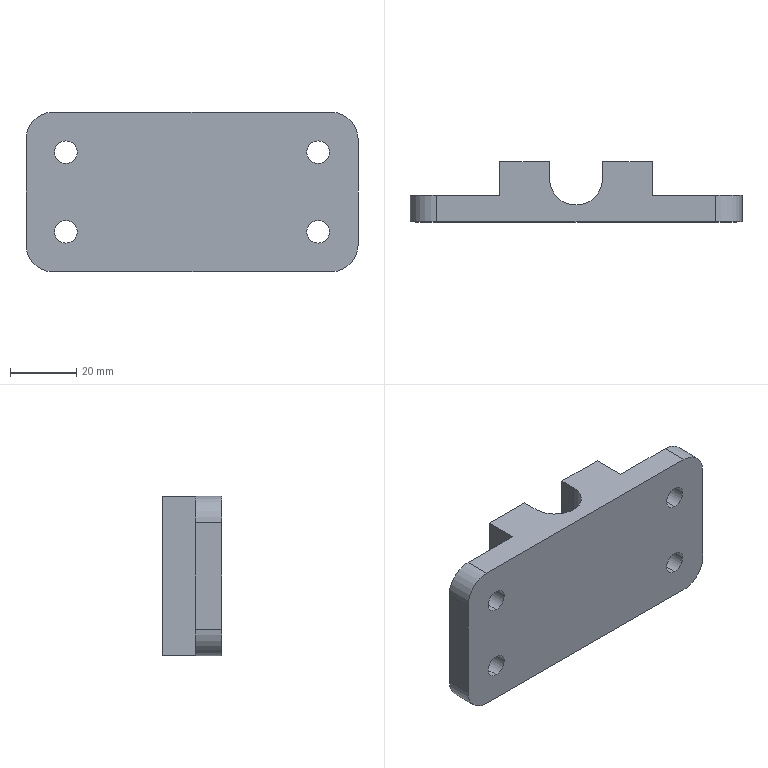Part | SolidWorks | features HoleWzd 2, ICE 2, Extrusion 1, Fillet 1 | 1 solid | 42 faces | box 100 x 18 x 48 mm | volume 49859 mm3 | cylinder 21 | plane 13 | cone 8 | commonest cylinder face diameters 3.3 x8 6.8 x8 16 x5
STEP:
#1=CARTESIAN_POINT('',(-38.,0.,-15.4));
#2=VERTEX_POINT('',#1);
#3=CARTESIAN_POINT('',(-38.,0.,-8.6));
#4=VERTEX_POINT('',#3);
#5=CARTESIAN_POINT('',(-38.,0.,-12.));
#6=DIRECTION('',(0.,1.,0.));
#7=DIRECTION('',(0.,0.,1.));
#8=AXIS2_PLACEMENT_3D('',#5,#6,#7);
#9=CIRCLE('',#8,3.4);
#10=EDGE_CURVE('',#2,#4,#9,.T.);
#11=ORIENTED_EDGE('',*,*,#10,.F.);
#12=CARTESIAN_POINT('',(-38.,8.,-15.4));
#13=VERTEX_POINT('',#12);
#14=CARTESIAN_POINT('',(-38.,8.,-15.4));
#15=DIRECTION('',(0.,1.,0.));
#16=VECTOR('',#15,1000.);
#17=LINE('',#14,#16);
#18=EDGE_CURVE('',#2,#13,#17,.T.);
#19=ORIENTED_EDGE('',*,*,#18,.T.);
#20=CARTESIAN_POINT('',(-38.,8.,-8.6));
#21=VERTEX_POINT('',#20);
#22=CARTESIAN_POINT('',(-38.,8.,-12.));
#23=DIRECTION('',(0.,1.,0.));
#24=DIRECTION('',(0.,0.,1.));
#25=AXIS2_PLACEMENT_3D('',#22,#23,#24);
#26=CIRCLE('',#25,3.4);
#27=EDGE_CURVE('',#13,#21,#26,.T.);
#28=ORIENTED_EDGE('',*,*,#27,.T.);
#29=CARTESIAN_POINT('',(-38.,8.,-8.6));
#30=DIRECTION('',(0.,1.,0.));
#31=VECTOR('',#30,1000.);
#32=LINE('',#29,#31);
#33=EDGE_CURVE('',#4,#21,#32,.T.);
#34=ORIENTED_EDGE('',*,*,#33,.F.);
#35=EDGE_LOOP('',(#11,#19,#28,#34));
#36=FACE_OUTER_BOUND('',#35,.T.);
#37=CARTESIAN_POINT('',(-38.,8.,-12.));
#38=DIRECTION('',(0.,1.,0.));
#39=DIRECTION('',(0.,0.,1.));
#40=AXIS2_PLACEMENT_3D('',#37,#38,#39);
#41=CYLINDRICAL_SURFACE('',#40,3.4);
#42=ADVANCED_FACE('',(#36),#41,.F.);
#43=CARTESIAN_POINT('',(-38.,0.,8.6));
#44=VERTEX_POINT('',#43);
#45=CARTESIAN_POINT('',(-38.,0.,15.4));
#46=VERTEX_POINT('',#45);
#47=CARTESIAN_POINT('',(-38.,0.,12.));
#48=DIRECTION('',(0.,1.,0.));
#49=DIRECTION('',(0.,0.,1.));
#50=AXIS2_PLACEMENT_3D('',#47,#48,#49);
#51=CIRCLE('',#50,3.4);
#52=EDGE_CURVE('',#44,#46,#51,.T.);
#53=ORIENTED_EDGE('',*,*,#52,.F.);
#54=CARTESIAN_POINT('',(-38.,8.,8.6));
#55=VERTEX_POINT('',#54);
#56=CARTESIAN_POINT('',(-38.,8.,8.6));
#57=DIRECTION('',(0.,1.,0.));
#58=VECTOR('',#57,1000.);
#59=LINE('',#56,#58);
#60=EDGE_CURVE('',#44,#55,#59,.T.);
#61=ORIENTED_EDGE('',*,*,#60,.T.);
#62=CARTESIAN_POINT('',(-38.,8.,15.4));
#63=VERTEX_POINT('',#62);
#64=CARTESIAN_POINT('',(-38.,8.,12.));
#65=DIRECTION('',(0.,1.,0.));
#66=DIRECTION('',(0.,0.,1.));
#67=AXIS2_PLACEMENT_3D('',#64,#65,#66);
#68=CIRCLE('',#67,3.4);
#69=EDGE_CURVE('',#55,#63,#68,.T.);
#70=ORIENTED_EDGE('',*,*,#69,.T.);
#71=CARTESIAN_POINT('',(-38.,8.,15.4));
#72=DIRECTION('',(0.,1.,0.));
#73=VECTOR('',#72,1000.);
#74=LINE('',#71,#73);
#75=EDGE_CURVE('',#46,#63,#74,.T.);
#76=ORIENTED_EDGE('',*,*,#75,.F.);
#77=EDGE_LOOP('',(#53,#61,#70,#76));
#78=FACE_OUTER_BOUND('',#77,.T.);
#79=CARTESIAN_POINT('',(-38.,8.,12.));
#80=DIRECTION('',(0.,1.,0.));
#81=DIRECTION('',(0.,0.,1.));
#82=AXIS2_PLACEMENT_3D('',#79,#80,#81);
#83=CYLINDRICAL_SURFACE('',#82,3.4);
#84=ADVANCED_FACE('',(#78),#83,.F.);
#85=CARTESIAN_POINT('',(38.,0.,8.6));
#86=VERTEX_POINT('',#85);
#87=CARTESIAN_POINT('',(38.,0.,15.4));
#88=VERTEX_POINT('',#87);
#89=CARTESIAN_POINT('',(38.,0.,12.));
#90=DIRECTION('',(0.,1.,0.));
#91=DIRECTION('',(0.,0.,1.));
#92=AXIS2_PLACEMENT_3D('',#89,#90,#91);
#93=CIRCLE('',#92,3.4);
#94=EDGE_CURVE('',#86,#88,#93,.T.);
#95=ORIENTED_EDGE('',*,*,#94,.F.);
#96=CARTESIAN_POINT('',(38.,8.,8.6));
#97=VERTEX_POINT('',#96);
#98=CARTESIAN_POINT('',(38.,8.,8.6));
#99=DIRECTION('',(0.,1.,0.));
#100=VECTOR('',#99,1000.);
#101=LINE('',#98,#100);
#102=EDGE_CURVE('',#86,#97,#101,.T.);
#103=ORIENTED_EDGE('',*,*,#102,.T.);
#104=CARTESIAN_POINT('',(38.,8.,15.4));
#105=VERTEX_POINT('',#104);
#106=CARTESIAN_POINT('',(38.,8.,12.));
#107=DIRECTION('',(0.,1.,0.));
#108=DIRECTION('',(0.,0.,1.));
#109=AXIS2_PLACEMENT_3D('',#106,#107,#108);
#110=CIRCLE('',#109,3.4);
#111=EDGE_CURVE('',#97,#105,#110,.T.);
#112=ORIENTED_EDGE('',*,*,#111,.T.);
#113=CARTESIAN_POINT('',(38.,8.,15.4));
#114=DIRECTION('',(0.,1.,0.));
#115=VECTOR('',#114,1000.);
#116=LINE('',#113,#115);
#117=EDGE_CURVE('',#88,#105,#116,.T.);
#118=ORIENTED_EDGE('',*,*,#117,.F.);
#119=EDGE_LOOP('',(#95,#103,#112,#118));
#120=FACE_OUTER_BOUND('',#119,.T.);
#121=CARTESIAN_POINT('',(38.,8.,12.));
#122=DIRECTION('',(0.,1.,0.));
#123=DIRECTION('',(0.,0.,1.));
#124=AXIS2_PLACEMENT_3D('',#121,#122,#123);
#125=CYLINDRICAL_SURFACE('',#124,3.4);
#126=ADVANCED_FACE('',(#120),#125,.F.);
#127=CARTESIAN_POINT('',(38.,0.,-15.4));
#128=VERTEX_POINT('',#127);
#129=CARTESIAN_POINT('',(38.,0.,-8.6));
#130=VERTEX_POINT('',#129);
#131=CARTESIAN_POINT('',(38.,0.,-12.));
#132=DIRECTION('',(0.,1.,0.));
#133=DIRECTION('',(0.,0.,1.));
#134=AXIS2_PLACEMENT_3D('',#131,#132,#133);
#135=CIRCLE('',#134,3.4);
#136=EDGE_CURVE('',#128,#130,#135,.T.);
#137=ORIENTED_EDGE('',*,*,#136,.F.);
#138=CARTESIAN_POINT('',(38.,8.,-15.4));
#139=VERTEX_POINT('',#138);
#140=CARTESIAN_POINT('',(38.,8.,-15.4));
#141=DIRECTION('',(0.,1.,0.));
#142=VECTOR('',#141,1000.);
#143=LINE('',#140,#142);
#144=EDGE_CURVE('',#128,#139,#143,.T.);
#145=ORIENTED_EDGE('',*,*,#144,.T.);
#146=CARTESIAN_POINT('',(38.,8.,-8.6));
#147=VERTEX_POINT('',#146);
#148=CARTESIAN_POINT('',(38.,8.,-12.));
#149=DIRECTION('',(0.,1.,0.));
#150=DIRECTION('',(0.,0.,1.));
#151=AXIS2_PLACEMENT_3D('',#148,#149,#150);
#152=CIRCLE('',#151,3.4);
#153=EDGE_CURVE('',#139,#147,#152,.T.);
#154=ORIENTED_EDGE('',*,*,#153,.T.);
#155=CARTESIAN_POINT('',(38.,8.,-8.6));
#156=DIRECTION('',(0.,1.,0.));
#157=VECTOR('',#156,1000.);
#158=LINE('',#155,#157);
#159=EDGE_CURVE('',#130,#147,#158,.T.);
#160=ORIENTED_EDGE('',*,*,#159,.F.);
#161=EDGE_LOOP('',(#137,#145,#154,#160));
#162=FACE_OUTER_BOUND('',#161,.T.);
#163=CARTESIAN_POINT('',(38.,8.,-12.));
#164=DIRECTION('',(0.,1.,0.));
#165=DIRECTION('',(0.,0.,1.));
#166=AXIS2_PLACEMENT_3D('',#163,#164,#165);
#167=CYLINDRICAL_SURFACE('',#166,3.4);
#168=ADVANCED_FACE('',(#162),#167,.F.);
#169=CARTESIAN_POINT('',(-15.,8.,-15.65));
#170=VERTEX_POINT('',#169);
#171=CARTESIAN_POINT('',(-15.,8.,-12.35));
#172=VERTEX_POINT('',#171);
#173=CARTESIAN_POINT('',(-15.,8.,-14.));
#174=DIRECTION('',(0.,1.,0.));
#175=DIRECTION('',(0.,0.,1.));
#176=AXIS2_PLACEMENT_3D('',#173,#174,#175);
#177=CIRCLE('',#176,1.65);
#178=EDGE_CURVE('',#170,#172,#177,.T.);
#179=ORIENTED_EDGE('',*,*,#178,.F.);
#180=CARTESIAN_POINT('',(-15.,18.,-15.65));
#181=VERTEX_POINT('',#180);
#182=CARTESIAN_POINT('',(-15.,18.,-15.65));
#183=DIRECTION('',(0.,1.,0.));
#184=VECTOR('',#183,1000.);
#185=LINE('',#182,#184);
#186=EDGE_CURVE('',#170,#181,#185,.T.);
#187=ORIENTED_EDGE('',*,*,#186,.T.);
#188=CARTESIAN_POINT('',(-15.,18.,-12.35));
#189=VERTEX_POINT('',#188);
#190=CARTESIAN_POINT('',(-15.,18.,-14.));
#191=DIRECTION('',(0.,1.,0.));
#192=DIRECTION('',(0.,0.,1.));
#193=AXIS2_PLACEMENT_3D('',#190,#191,#192);
#194=CIRCLE('',#193,1.65);
#195=EDGE_CURVE('',#181,#189,#194,.T.);
#196=ORIENTED_EDGE('',*,*,#195,.T.);
#197=CARTESIAN_POINT('',(-15.,18.,-12.35));
#198=DIRECTION('',(0.,1.,0.));
#199=VECTOR('',#198,1000.);
#200=LINE('',#197,#199);
#201=EDGE_CURVE('',#172,#189,#200,.T.);
#202=ORIENTED_EDGE('',*,*,#201,.F.);
#203=EDGE_LOOP('',(#179,#187,#196,#202));
#204=FACE_OUTER_BOUND('',#203,.T.);
#205=CARTESIAN_POINT('',(-15.,18.,-14.));
#206=DIRECTION('',(0.,1.,0.));
#207=DIRECTION('',(0.,0.,1.));
#208=AXIS2_PLACEMENT_3D('',#205,#206,#207);
#209=CYLINDRICAL_SURFACE('',#208,1.65);
#210=ADVANCED_FACE('',(#204),#209,.F.);
#211=CARTESIAN_POINT('',(-15.,7.009,-14.));
#212=VERTEX_POINT('',#211);
#213=CARTESIAN_POINT('',(-15.,8.,-12.35));
#214=DIRECTION('',(0.,0.515,0.8572));
#215=VECTOR('',#214,1000.);
#216=LINE('',#213,#215);
#217=EDGE_CURVE('',#212,#172,#216,.T.);
#218=ORIENTED_EDGE('',*,*,#217,.F.);
#219=CARTESIAN_POINT('',(-15.,8.,-15.65));
#220=DIRECTION('',(0.,0.515,-0.8572));
#221=VECTOR('',#220,1000.);
#222=LINE('',#219,#221);
#223=EDGE_CURVE('',#212,#170,#222,.T.);
#224=ORIENTED_EDGE('',*,*,#223,.T.);
#225=ORIENTED_EDGE('',*,*,#178,.T.);
#226=EDGE_LOOP('',(#218,#224,#225));
#227=FACE_OUTER_BOUND('',#226,.T.);
#228=CARTESIAN_POINT('',(-15.,8.,-14.));
#229=DIRECTION('',(0.,1.,0.));
#230=DIRECTION('',(0.,0.,1.));
#231=AXIS2_PLACEMENT_3D('',#228,#229,#230);
#232=CONICAL_SURFACE('',#231,1.65,1.03);
#233=ADVANCED_FACE('',(#227),#232,.F.);
#234=CARTESIAN_POINT('',(-15.,8.,12.35));
#235=VERTEX_POINT('',#234);
#236=CARTESIAN_POINT('',(-15.,8.,15.65));
#237=VERTEX_POINT('',#236);
#238=CARTESIAN_POINT('',(-15.,8.,14.));
#239=DIRECTION('',(0.,1.,0.));
#240=DIRECTION('',(0.,0.,1.));
#241=AXIS2_PLACEMENT_3D('',#238,#239,#240);
#242=CIRCLE('',#241,1.65);
#243=EDGE_CURVE('',#235,#237,#242,.T.);
#244=ORIENTED_EDGE('',*,*,#243,.F.);
#245=CARTESIAN_POINT('',(-15.,18.,12.35));
#246=VERTEX_POINT('',#245);
#247=CARTESIAN_POINT('',(-15.,18.,12.35));
#248=DIRECTION('',(0.,1.,0.));
#249=VECTOR('',#248,1000.);
#250=LINE('',#247,#249);
#251=EDGE_CURVE('',#235,#246,#250,.T.);
#252=ORIENTED_EDGE('',*,*,#251,.T.);
#253=CARTESIAN_POINT('',(-15.,18.,15.65));
#254=VERTEX_POINT('',#253);
#255=CARTESIAN_POINT('',(-15.,18.,14.));
#256=DIRECTION('',(0.,1.,0.));
#257=DIRECTION('',(0.,0.,1.));
#258=AXIS2_PLACEMENT_3D('',#255,#256,#257);
#259=CIRCLE('',#258,1.65);
#260=EDGE_CURVE('',#246,#254,#259,.T.);
#261=ORIENTED_EDGE('',*,*,#260,.T.);
#262=CARTESIAN_POINT('',(-15.,18.,15.65));
#263=DIRECTION('',(0.,1.,0.));
#264=VECTOR('',#263,1000.);
#265=LINE('',#262,#264);
#266=EDGE_CURVE('',#237,#254,#265,.T.);
#267=ORIENTED_EDGE('',*,*,#266,.F.);
#268=EDGE_LOOP('',(#244,#252,#261,#267));
#269=FACE_OUTER_BOUND('',#268,.T.);
#270=CARTESIAN_POINT('',(-15.,18.,14.));
#271=DIRECTION('',(0.,1.,0.));
#272=DIRECTION('',(0.,0.,1.));
#273=AXIS2_PLACEMENT_3D('',#270,#271,#272);
#274=CYLINDRICAL_SURFACE('',#273,1.65);
#275=ADVANCED_FACE('',(#269),#274,.F.);
#276=CARTESIAN_POINT('',(-15.,7.009,14.));
#277=VERTEX_POINT('',#276);
#278=CARTESIAN_POINT('',(-15.,8.,15.65));
#279=DIRECTION('',(0.,0.515,0.8572));
#280=VECTOR('',#279,1000.);
#281=LINE('',#278,#280);
#282=EDGE_CURVE('',#277,#237,#281,.T.);
#283=ORIENTED_EDGE('',*,*,#282,.F.);
#284=CARTESIAN_POINT('',(-15.,8.,12.35));
#285=DIRECTION('',(0.,0.515,-0.8572));
#286=VECTOR('',#285,1000.);
#287=LINE('',#284,#286);
#288=EDGE_CURVE('',#277,#235,#287,.T.);
#289=ORIENTED_EDGE('',*,*,#288,.T.);
#290=ORIENTED_EDGE('',*,*,#243,.T.);
#291=EDGE_LOOP('',(#283,#289,#290));
#292=FACE_OUTER_BOUND('',#291,.T.);
#293=CARTESIAN_POINT('',(-15.,8.,14.));
#294=DIRECTION('',(0.,1.,0.));
#295=DIRECTION('',(0.,0.,1.));
#296=AXIS2_PLACEMENT_3D('',#293,#294,#295);
#297=CONICAL_SURFACE('',#296,1.65,1.03);
#298=ADVANCED_FACE('',(#292),#297,.F.);
#299=CARTESIAN_POINT('',(15.,8.,12.35));
#300=VERTEX_POINT('',#299);
#301=CARTESIAN_POINT('',(15.,8.,15.65));
#302=VERTEX_POINT('',#301);
#303=CARTESIAN_POINT('',(15.,8.,14.));
#304=DIRECTION('',(0.,1.,0.));
#305=DIRECTION('',(0.,0.,1.));
#306=AXIS2_PLACEMENT_3D('',#303,#304,#305);
#307=CIRCLE('',#306,1.65);
#308=EDGE_CURVE('',#300,#302,#307,.T.);
#309=ORIENTED_EDGE('',*,*,#308,.F.);
#310=CARTESIAN_POINT('',(15.,18.,12.35));
#311=VERTEX_POINT('',#310);
#312=CARTESIAN_POINT('',(15.,18.,12.35));
#313=DIRECTION('',(0.,1.,0.));
#314=VECTOR('',#313,1000.);
#315=LINE('',#312,#314);
#316=EDGE_CURVE('',#300,#311,#315,.T.);
#317=ORIENTED_EDGE('',*,*,#316,.T.);
#318=CARTESIAN_POINT('',(15.,18.,15.65));
#319=VERTEX_POINT('',#318);
#320=CARTESIAN_POINT('',(15.,18.,14.));
#321=DIRECTION('',(0.,1.,0.));
#322=DIRECTION('',(0.,0.,1.));
#323=AXIS2_PLACEMENT_3D('',#320,#321,#322);
#324=CIRCLE('',#323,1.65);
#325=EDGE_CURVE('',#311,#319,#324,.T.);
#326=ORIENTED_EDGE('',*,*,#325,.T.);
#327=CARTESIAN_POINT('',(15.,18.,15.65));
#328=DIRECTION('',(0.,1.,0.));
#329=VECTOR('',#328,1000.);
#330=LINE('',#327,#329);
#331=EDGE_CURVE('',#302,#319,#330,.T.);
#332=ORIENTED_EDGE('',*,*,#331,.F.);
#333=EDGE_LOOP('',(#309,#317,#326,#332));
#334=FACE_OUTER_BOUND('',#333,.T.);
#335=CARTESIAN_POINT('',(15.,18.,14.));
#336=DIRECTION('',(0.,1.,0.));
#337=DIRECTION('',(0.,0.,1.));
#338=AXIS2_PLACEMENT_3D('',#335,#336,#337);
#339=CYLINDRICAL_SURFACE('',#338,1.65);
#340=ADVANCED_FACE('',(#334),#339,.F.);
#341=CARTESIAN_POINT('',(15.,7.009,14.));
#342=VERTEX_POINT('',#341);
#343=CARTESIAN_POINT('',(15.,8.,15.65));
#344=DIRECTION('',(0.,0.515,0.8572));
#345=VECTOR('',#344,1000.);
#346=LINE('',#343,#345);
#347=EDGE_CURVE('',#342,#302,#346,.T.);
#348=ORIENTED_EDGE('',*,*,#347,.F.);
#349=CARTESIAN_POINT('',(15.,8.,12.35));
#350=DIRECTION('',(0.,0.515,-0.8572));
#351=VECTOR('',#350,1000.);
#352=LINE('',#349,#351);
#353=EDGE_CURVE('',#342,#300,#352,.T.);
#354=ORIENTED_EDGE('',*,*,#353,.T.);
#355=ORIENTED_EDGE('',*,*,#308,.T.);
#356=EDGE_LOOP('',(#348,#354,#355));
#357=FACE_OUTER_BOUND('',#356,.T.);
#358=CARTESIAN_POINT('',(15.,8.,14.));
#359=DIRECTION('',(0.,1.,0.));
#360=DIRECTION('',(0.,0.,1.));
#361=AXIS2_PLACEMENT_3D('',#358,#359,#360);
#362=CONICAL_SURFACE('',#361,1.65,1.03);
#363=ADVANCED_FACE('',(#357),#362,.F.);
#364=CARTESIAN_POINT('',(15.,8.,-15.65));
#365=VERTEX_POINT('',#364);
#366=CARTESIAN_POINT('',(15.,8.,-12.35));
#367=VERTEX_POINT('',#366);
#368=CARTESIAN_POINT('',(15.,8.,-14.));
#369=DIRECTION('',(0.,1.,0.));
#370=DIRECTION('',(0.,0.,1.));
#371=AXIS2_PLACEMENT_3D('',#368,#369,#370);
#372=CIRCLE('',#371,1.65);
#373=EDGE_CURVE('',#365,#367,#372,.T.);
#374=ORIENTED_EDGE('',*,*,#373,.F.);
#375=CARTESIAN_POINT('',(15.,18.,-15.65));
#376=VERTEX_POINT('',#375);
#377=CARTESIAN_POINT('',(15.,18.,-15.65));
#378=DIRECTION('',(0.,1.,0.));
#379=VECTOR('',#378,1000.);
#380=LINE('',#377,#379);
#381=EDGE_CURVE('',#365,#376,#380,.T.);
#382=ORIENTED_EDGE('',*,*,#381,.T.);
#383=CARTESIAN_POINT('',(15.,18.,-12.35));
#384=VERTEX_POINT('',#383);
#385=CARTESIAN_POINT('',(15.,18.,-14.));
#386=DIRECTION('',(0.,1.,0.));
#387=DIRECTION('',(0.,0.,1.));
#388=AXIS2_PLACEMENT_3D('',#385,#386,#387);
#389=CIRCLE('',#388,1.65);
#390=EDGE_CURVE('',#376,#384,#389,.T.);
#391=ORIENTED_EDGE('',*,*,#390,.T.);
#392=CARTESIAN_POINT('',(15.,18.,-12.35));
#393=DIRECTION('',(0.,1.,0.));
#394=VECTOR('',#393,1000.);
#395=LINE('',#392,#394);
#396=EDGE_CURVE('',#367,#384,#395,.T.);
#397=ORIENTED_EDGE('',*,*,#396,.F.);
#398=EDGE_LOOP('',(#374,#382,#391,#397));
#399=FACE_OUTER_BOUND('',#398,.T.);
#400=CARTESIAN_POINT('',(15.,18.,-14.));
#401=DIRECTION('',(0.,1.,0.));
#402=DIRECTION('',(0.,0.,1.));
#403=AXIS2_PLACEMENT_3D('',#400,#401,#402);
#404=CYLINDRICAL_SURFACE('',#403,1.65);
#405=ADVANCED_FACE('',(#399),#404,.F.);
#406=CARTESIAN_POINT('',(15.,7.009,-14.));
#407=VERTEX_POINT('',#406);
#408=CARTESIAN_POINT('',(15.,8.,-12.35));
#409=DIRECTION('',(0.,0.515,0.8572));
#410=VECTOR('',#409,1000.);
#411=LINE('',#408,#410);
#412=EDGE_CURVE('',#407,#367,#411,.T.);
#413=ORIENTED_EDGE('',*,*,#412,.F.);
#414=CARTESIAN_POINT('',(15.,8.,-15.65));
#415=DIRECTION('',(0.,0.515,-0.8572));
#416=VECTOR('',#415,1000.);
#417=LINE('',#414,#416);
#418=EDGE_CURVE('',#407,#365,#417,.T.);
#419=ORIENTED_EDGE('',*,*,#418,.T.);
#420=ORIENTED_EDGE('',*,*,#373,.T.);
#421=EDGE_LOOP('',(#413,#419,#420));
#422=FACE_OUTER_BOUND('',#421,.T.);
#423=CARTESIAN_POINT('',(15.,8.,-14.));
#424=DIRECTION('',(0.,1.,0.));
#425=DIRECTION('',(0.,0.,1.));
#426=AXIS2_PLACEMENT_3D('',#423,#424,#425);
#427=CONICAL_SURFACE('',#426,1.65,1.03);
#428=ADVANCED_FACE('',(#422),#427,.F.);
#429=CARTESIAN_POINT('',(-15.,18.,-14.));
#430=DIRECTION('',(0.,1.,0.));
#431=DIRECTION('',(0.,0.,1.));
#432=AXIS2_PLACEMENT_3D('',#429,#430,#431);
#433=CIRCLE('',#432,1.65);
#434=EDGE_CURVE('',#189,#181,#433,.T.);
#435=ORIENTED_EDGE('',*,*,#434,.F.);
#436=ORIENTED_EDGE('',*,*,#195,.F.);
#437=EDGE_LOOP('',(#435,#436));
#438=FACE_BOUND('',#437,.T.);
#439=CARTESIAN_POINT('',(-15.,18.,14.));
#440=DIRECTION('',(0.,1.,0.));
#441=DIRECTION('',(0.,0.,1.));
#442=AXIS2_PLACEMENT_3D('',#439,#440,#441);
#443=CIRCLE('',#442,1.65);
#444=EDGE_CURVE('',#254,#246,#443,.T.);
#445=ORIENTED_EDGE('',*,*,#444,.F.);
#446=ORIENTED_EDGE('',*,*,#260,.F.);
#447=EDGE_LOOP('',(#445,#446));
#448=FACE_BOUND('',#447,.T.);
#449=CARTESIAN_POINT('',(-8.,18.,-24.));
#450=VERTEX_POINT('',#449);
#451=CARTESIAN_POINT('',(-8.,18.,24.));
#452=VERTEX_POINT('',#451);
#453=CARTESIAN_POINT('',(-8.,18.,-24.));
#454=DIRECTION('',(0.,0.,1.));
#455=VECTOR('',#454,1000.);
#456=LINE('',#453,#455);
#457=EDGE_CURVE('',#450,#452,#456,.T.);
#458=ORIENTED_EDGE('',*,*,#457,.F.);
#459=CARTESIAN_POINT('',(-23.,18.,-24.));
#460=VERTEX_POINT('',#459);
#461=CARTESIAN_POINT('',(-23.,18.,-24.));
#462=DIRECTION('',(-1.,0.,0.));
#463=VECTOR('',#462,1000.);
#464=LINE('',#461,#463);
#465=EDGE_CURVE('',#450,#460,#464,.T.);
#466=ORIENTED_EDGE('',*,*,#465,.T.);
#467=CARTESIAN_POINT('',(-23.,18.,24.));
#468=VERTEX_POINT('',#467);
#469=CARTESIAN_POINT('',(-23.,18.,-24.));
#470=DIRECTION('',(0.,0.,1.));
#471=VECTOR('',#470,1000.);
#472=LINE('',#469,#471);
#473=EDGE_CURVE('',#460,#468,#472,.T.);
#474=ORIENTED_EDGE('',*,*,#473,.T.);
#475=CARTESIAN_POINT('',(-23.,18.,24.));
#476=DIRECTION('',(1.,0.,0.));
#477=VECTOR('',#476,1000.);
#478=LINE('',#475,#477);
#479=EDGE_CURVE('',#468,#452,#478,.T.);
#480=ORIENTED_EDGE('',*,*,#479,.T.);
#481=EDGE_LOOP('',(#458,#466,#474,#480));
#482=FACE_OUTER_BOUND('',#481,.T.);
#483=CARTESIAN_POINT('',(0.,18.,0.));
#484=DIRECTION('',(0.,1.,0.));
#485=DIRECTION('',(0.,0.,1.));
#486=AXIS2_PLACEMENT_3D('',#483,#484,#485);
#487=PLANE('',#486);
#488=ADVANCED_FACE('',(#438,#448,#482),#487,.T.);
#489=CARTESIAN_POINT('',(38.,8.,12.));
#490=DIRECTION('',(0.,1.,0.));
#491=DIRECTION('',(0.,0.,1.));
#492=AXIS2_PLACEMENT_3D('',#489,#490,#491);
#493=CIRCLE('',#492,3.4);
#494=EDGE_CURVE('',#105,#97,#493,.T.);
#495=ORIENTED_EDGE('',*,*,#494,.F.);
#496=ORIENTED_EDGE('',*,*,#111,.F.);
#497=EDGE_LOOP('',(#495,#496));
#498=FACE_BOUND('',#497,.T.);
#499=CARTESIAN_POINT('',(38.,8.,-12.));
#500=DIRECTION('',(0.,1.,0.));
#501=DIRECTION('',(0.,0.,1.));
#502=AXIS2_PLACEMENT_3D('',#499,#500,#501);
#503=CIRCLE('',#502,3.4);
#504=EDGE_CURVE('',#147,#139,#503,.T.);
#505=ORIENTED_EDGE('',*,*,#504,.F.);
#506=ORIENTED_EDGE('',*,*,#153,.F.);
#507=EDGE_LOOP('',(#505,#506));
#508=FACE_BOUND('',#507,.T.);
#509=CARTESIAN_POINT('',(50.,8.,16.));
#510=VERTEX_POINT('',#509);
#511=CARTESIAN_POINT('',(50.,8.,-16.));
#512=VERTEX_POINT('',#511);
#513=CARTESIAN_POINT('',(50.,8.,-24.));
#514=DIRECTION('',(0.,0.,-1.));
#515=VECTOR('',#514,1000.);
#516=LINE('',#513,#515);
#517=EDGE_CURVE('',#510,#512,#516,.T.);
#518=ORIENTED_EDGE('',*,*,#517,.T.);
#519=CARTESIAN_POINT('',(42.,8.,-24.));
#520=VERTEX_POINT('',#519);
#521=CARTESIAN_POINT('',(42.,8.,-16.));
#522=DIRECTION('',(0.,1.,0.));
#523=DIRECTION('',(0.,0.,1.));
#524=AXIS2_PLACEMENT_3D('',#521,#522,#523);
#525=CIRCLE('',#524,8.);
#526=EDGE_CURVE('',#512,#520,#525,.T.);
#527=ORIENTED_EDGE('',*,*,#526,.T.);
#528=CARTESIAN_POINT('',(23.,8.,-24.));
#529=VERTEX_POINT('',#528);
#530=CARTESIAN_POINT('',(-50.,8.,-24.));
#531=DIRECTION('',(-1.,0.,0.));
#532=VECTOR('',#531,1000.);
#533=LINE('',#530,#532);
#534=EDGE_CURVE('',#520,#529,#533,.T.);
#535=ORIENTED_EDGE('',*,*,#534,.T.);
#536=CARTESIAN_POINT('',(23.,8.,24.));
#537=VERTEX_POINT('',#536);
#538=CARTESIAN_POINT('',(23.,8.,-24.));
#539=DIRECTION('',(0.,0.,-1.));
#540=VECTOR('',#539,1000.);
#541=LINE('',#538,#540);
#542=EDGE_CURVE('',#537,#529,#541,.T.);
#543=ORIENTED_EDGE('',*,*,#542,.F.);
#544=CARTESIAN_POINT('',(42.,8.,24.));
#545=VERTEX_POINT('',#544);
#546=CARTESIAN_POINT('',(-50.,8.,24.));
#547=DIRECTION('',(1.,0.,0.));
#548=VECTOR('',#547,1000.);
#549=LINE('',#546,#548);
#550=EDGE_CURVE('',#537,#545,#549,.T.);
#551=ORIENTED_EDGE('',*,*,#550,.T.);
#552=CARTESIAN_POINT('',(42.,8.,16.));
#553=DIRECTION('',(0.,1.,0.));
#554=DIRECTION('',(0.,0.,1.));
#555=AXIS2_PLACEMENT_3D('',#552,#553,#554);
#556=CIRCLE('',#555,8.);
#557=EDGE_CURVE('',#545,#510,#556,.T.);
#558=ORIENTED_EDGE('',*,*,#557,.T.);
#559=EDGE_LOOP('',(#518,#527,#535,#543,#551,#558));
#560=FACE_OUTER_BOUND('',#559,.T.);
#561=CARTESIAN_POINT('',(0.,8.,0.));
#562=DIRECTION('',(0.,1.,0.));
#563=DIRECTION('',(0.,0.,1.));
#564=AXIS2_PLACEMENT_3D('',#561,#562,#563);
#565=PLANE('',#564);
#566=ADVANCED_FACE('',(#498,#508,#560),#565,.T.);
#567=CARTESIAN_POINT('',(50.,0.,16.));
#568=VERTEX_POINT('',#567);
#569=CARTESIAN_POINT('',(50.,0.,-16.));
#570=VERTEX_POINT('',#569);
#571=CARTESIAN_POINT('',(50.,0.,-24.));
#572=DIRECTION('',(0.,0.,-1.));
#573=VECTOR('',#572,1000.);
#574=LINE('',#571,#573);
#575=EDGE_CURVE('',#568,#570,#574,.T.);
#576=ORIENTED_EDGE('',*,*,#575,.T.);
#577=CARTESIAN_POINT('',(50.,8.,-16.));
#578=DIRECTION('',(0.,1.,0.));
#579=VECTOR('',#578,1000.);
#580=LINE('',#577,#579);
#581=EDGE_CURVE('',#570,#512,#580,.T.);
#582=ORIENTED_EDGE('',*,*,#581,.T.);
#583=ORIENTED_EDGE('',*,*,#517,.F.);
#584=CARTESIAN_POINT('',(50.,8.,16.));
#585=DIRECTION('',(0.,-1.,0.));
#586=VECTOR('',#585,1000.);
#587=LINE('',#584,#586);
#588=EDGE_CURVE('',#510,#568,#587,.T.);
#589=ORIENTED_EDGE('',*,*,#588,.T.);
#590=EDGE_LOOP('',(#576,#582,#583,#589));
#591=FACE_OUTER_BOUND('',#590,.T.);
#592=CARTESIAN_POINT('',(50.,8.,-24.));
#593=DIRECTION('',(-1.,0.,0.));
#594=DIRECTION('',(0.,0.,1.));
#595=AXIS2_PLACEMENT_3D('',#592,#593,#594);
#596=PLANE('',#595);
#597=ADVANCED_FACE('',(#591),#596,.F.);
#598=ORIENTED_EDGE('',*,*,#534,.F.);
#599=CARTESIAN_POINT('',(42.,0.,-24.));
#600=VERTEX_POINT('',#599);
#601=CARTESIAN_POINT('',(42.,8.,-24.));
#602=DIRECTION('',(0.,-1.,0.));
#603=VECTOR('',#602,1000.);
#604=LINE('',#601,#603);
#605=EDGE_CURVE('',#520,#600,#604,.T.);
#606=ORIENTED_EDGE('',*,*,#605,.T.);
#607=CARTESIAN_POINT('',(-42.,0.,-24.));
#608=VERTEX_POINT('',#607);
#609=CARTESIAN_POINT('',(-50.,0.,-24.));
#610=DIRECTION('',(-1.,0.,0.));
#611=VECTOR('',#610,1000.);
#612=LINE('',#609,#611);
#613=EDGE_CURVE('',#600,#608,#612,.T.);
#614=ORIENTED_EDGE('',*,*,#613,.T.);
#615=CARTESIAN_POINT('',(-42.,8.,-24.));
#616=VERTEX_POINT('',#615);
#617=CARTESIAN_POINT('',(-42.,8.,-24.));
#618=DIRECTION('',(0.,1.,0.));
#619=VECTOR('',#618,1000.);
#620=LINE('',#617,#619);
#621=EDGE_CURVE('',#608,#616,#620,.T.);
#622=ORIENTED_EDGE('',*,*,#621,.T.);
#623=CARTESIAN_POINT('',(-23.,8.,-24.));
#624=VERTEX_POINT('',#623);
#625=CARTESIAN_POINT('',(-50.,8.,-24.));
#626=DIRECTION('',(-1.,0.,0.));
#627=VECTOR('',#626,1000.);
#628=LINE('',#625,#627);
#629=EDGE_CURVE('',#624,#616,#628,.T.);
#630=ORIENTED_EDGE('',*,*,#629,.F.);
#631=CARTESIAN_POINT('',(-23.,18.,-24.));
#632=DIRECTION('',(0.,-1.,0.));
#633=VECTOR('',#632,1000.);
#634=LINE('',#631,#633);
#635=EDGE_CURVE('',#460,#624,#634,.T.);
#636=ORIENTED_EDGE('',*,*,#635,.F.);
#637=ORIENTED_EDGE('',*,*,#465,.F.);
#638=CARTESIAN_POINT('',(-8.,13.,-24.));
#639=VERTEX_POINT('',#638);
#640=CARTESIAN_POINT('',(-8.,13.,-24.));
#641=DIRECTION('',(0.,-1.,0.));
#642=VECTOR('',#641,1000.);
#643=LINE('',#640,#642);
#644=EDGE_CURVE('',#450,#639,#643,.T.);
#645=ORIENTED_EDGE('',*,*,#644,.T.);
#646=CARTESIAN_POINT('',(8.,13.,-24.));
#647=VERTEX_POINT('',#646);
#648=CARTESIAN_POINT('',(0.,13.,-24.));
#649=DIRECTION('',(0.,0.,1.));
#650=DIRECTION('',(1.,0.,0.));
#651=AXIS2_PLACEMENT_3D('',#648,#649,#650);
#652=CIRCLE('',#651,8.);
#653=EDGE_CURVE('',#639,#647,#652,.T.);
#654=ORIENTED_EDGE('',*,*,#653,.T.);
#655=CARTESIAN_POINT('',(8.,18.,-24.));
#656=VERTEX_POINT('',#655);
#657=CARTESIAN_POINT('',(8.,13.,-24.));
#658=DIRECTION('',(0.,1.,0.));
#659=VECTOR('',#658,1000.);
#660=LINE('',#657,#659);
#661=EDGE_CURVE('',#647,#656,#660,.T.);
#662=ORIENTED_EDGE('',*,*,#661,.T.);
#663=CARTESIAN_POINT('',(23.,18.,-24.));
#664=VERTEX_POINT('',#663);
#665=CARTESIAN_POINT('',(-23.,18.,-24.));
#666=DIRECTION('',(-1.,0.,0.));
#667=VECTOR('',#666,1000.);
#668=LINE('',#665,#667);
#669=EDGE_CURVE('',#664,#656,#668,.T.);
#670=ORIENTED_EDGE('',*,*,#669,.F.);
#671=CARTESIAN_POINT('',(23.,18.,-24.));
#672=DIRECTION('',(0.,-1.,0.));
#673=VECTOR('',#672,1000.);
#674=LINE('',#671,#673);
#675=EDGE_CURVE('',#664,#529,#674,.T.);
#676=ORIENTED_EDGE('',*,*,#675,.T.);
#677=EDGE_LOOP('',(#598,#606,#614,#622,#630,#636,#637,#645,#654,#662,#670,#676));
#678=FACE_OUTER_BOUND('',#677,.T.);
#679=CARTESIAN_POINT('',(-50.,8.,-24.));
#680=DIRECTION('',(0.,0.,1.));
#681=DIRECTION('',(1.,0.,0.));
#682=AXIS2_PLACEMENT_3D('',#679,#680,#681);
#683=PLANE('',#682);
#684=ADVANCED_FACE('',(#678),#683,.F.);
#685=CARTESIAN_POINT('',(-50.,8.,-16.));
#686=VERTEX_POINT('',#685);
#687=CARTESIAN_POINT('',(-50.,8.,16.));
#688=VERTEX_POINT('',#687);
#689=CARTESIAN_POINT('',(-50.,8.,-24.));
#690=DIRECTION('',(0.,0.,1.));
#691=VECTOR('',#690,1000.);
#692=LINE('',#689,#691);
#693=EDGE_CURVE('',#686,#688,#692,.T.);
#694=ORIENTED_EDGE('',*,*,#693,.F.);
#695=CARTESIAN_POINT('',(-50.,0.,-16.));
#696=VERTEX_POINT('',#695);
#697=CARTESIAN_POINT('',(-50.,8.,-16.));
#698=DIRECTION('',(0.,-1.,0.));
#699=VECTOR('',#698,1000.);
#700=LINE('',#697,#699);
#701=EDGE_CURVE('',#686,#696,#700,.T.);
#702=ORIENTED_EDGE('',*,*,#701,.T.);
#703=CARTESIAN_POINT('',(-50.,0.,16.));
#704=VERTEX_POINT('',#703);
#705=CARTESIAN_POINT('',(-50.,0.,-24.));
#706=DIRECTION('',(0.,0.,1.));
#707=VECTOR('',#706,1000.);
#708=LINE('',#705,#707);
#709=EDGE_CURVE('',#696,#704,#708,.T.);
#710=ORIENTED_EDGE('',*,*,#709,.T.);
#711=CARTESIAN_POINT('',(-50.,8.,16.));
#712=DIRECTION('',(0.,1.,0.));
#713=VECTOR('',#712,1000.);
#714=LINE('',#711,#713);
#715=EDGE_CURVE('',#704,#688,#714,.T.);
#716=ORIENTED_EDGE('',*,*,#715,.T.);
#717=EDGE_LOOP('',(#694,#702,#710,#716));
#718=FACE_OUTER_BOUND('',#717,.T.);
#719=CARTESIAN_POINT('',(-50.,8.,-24.));
#720=DIRECTION('',(1.,0.,0.));
#721=DIRECTION('',(0.,0.,-1.));
#722=AXIS2_PLACEMENT_3D('',#719,#720,#721);
#723=PLANE('',#722);
#724=ADVANCED_FACE('',(#718),#723,.F.);
#725=CARTESIAN_POINT('',(-42.,0.,24.));
#726=VERTEX_POINT('',#725);
#727=CARTESIAN_POINT('',(42.,0.,24.));
#728=VERTEX_POINT('',#727);
#729=CARTESIAN_POINT('',(-50.,0.,24.));
#730=DIRECTION('',(1.,0.,0.));
#731=VECTOR('',#730,1000.);
#732=LINE('',#729,#731);
#733=EDGE_CURVE('',#726,#728,#732,.T.);
#734=ORIENTED_EDGE('',*,*,#733,.T.);
#735=CARTESIAN_POINT('',(42.,8.,24.));
#736=DIRECTION('',(0.,1.,0.));
#737=VECTOR('',#736,1000.);
#738=LINE('',#735,#737);
#739=EDGE_CURVE('',#728,#545,#738,.T.);
#740=ORIENTED_EDGE('',*,*,#739,.T.);
#741=ORIENTED_EDGE('',*,*,#550,.F.);
#742=CARTESIAN_POINT('',(23.,18.,24.));
#743=VERTEX_POINT('',#742);
#744=CARTESIAN_POINT('',(23.,18.,24.));
#745=DIRECTION('',(0.,-1.,0.));
#746=VECTOR('',#745,1000.);
#747=LINE('',#744,#746);
#748=EDGE_CURVE('',#743,#537,#747,.T.);
#749=ORIENTED_EDGE('',*,*,#748,.F.);
#750=CARTESIAN_POINT('',(8.,18.,24.));
#751=VERTEX_POINT('',#750);
#752=CARTESIAN_POINT('',(-23.,18.,24.));
#753=DIRECTION('',(1.,0.,0.));
#754=VECTOR('',#753,1000.);
#755=LINE('',#752,#754);
#756=EDGE_CURVE('',#751,#743,#755,.T.);
#757=ORIENTED_EDGE('',*,*,#756,.F.);
#758=CARTESIAN_POINT('',(8.,13.,24.));
#759=VERTEX_POINT('',#758);
#760=CARTESIAN_POINT('',(8.,13.,24.));
#761=DIRECTION('',(0.,1.,0.));
#762=VECTOR('',#761,1000.);
#763=LINE('',#760,#762);
#764=EDGE_CURVE('',#759,#751,#763,.T.);
#765=ORIENTED_EDGE('',*,*,#764,.F.);
#766=CARTESIAN_POINT('',(-8.,13.,24.));
#767=VERTEX_POINT('',#766);
#768=CARTESIAN_POINT('',(0.,13.,24.));
#769=DIRECTION('',(0.,0.,1.));
#770=DIRECTION('',(1.,0.,0.));
#771=AXIS2_PLACEMENT_3D('',#768,#769,#770);
#772=CIRCLE('',#771,8.);
#773=EDGE_CURVE('',#767,#759,#772,.T.);
#774=ORIENTED_EDGE('',*,*,#773,.F.);
#775=CARTESIAN_POINT('',(-8.,13.,24.));
#776=DIRECTION('',(0.,-1.,0.));
#777=VECTOR('',#776,1000.);
#778=LINE('',#775,#777);
#779=EDGE_CURVE('',#452,#767,#778,.T.);
#780=ORIENTED_EDGE('',*,*,#779,.F.);
#781=ORIENTED_EDGE('',*,*,#479,.F.);
#782=CARTESIAN_POINT('',(-23.,8.,24.));
#783=VERTEX_POINT('',#782);
#784=CARTESIAN_POINT('',(-23.,18.,24.));
#785=DIRECTION('',(0.,-1.,0.));
#786=VECTOR('',#785,1000.);
#787=LINE('',#784,#786);
#788=EDGE_CURVE('',#468,#783,#787,.T.);
#789=ORIENTED_EDGE('',*,*,#788,.T.);
#790=CARTESIAN_POINT('',(-42.,8.,24.));
#791=VERTEX_POINT('',#790);
#792=CARTESIAN_POINT('',(-50.,8.,24.));
#793=DIRECTION('',(1.,0.,0.));
#794=VECTOR('',#793,1000.);
#795=LINE('',#792,#794);
#796=EDGE_CURVE('',#791,#783,#795,.T.);
#797=ORIENTED_EDGE('',*,*,#796,.F.);
#798=CARTESIAN_POINT('',(-42.,8.,24.));
#799=DIRECTION('',(0.,-1.,0.));
#800=VECTOR('',#799,1000.);
#801=LINE('',#798,#800);
#802=EDGE_CURVE('',#791,#726,#801,.T.);
#803=ORIENTED_EDGE('',*,*,#802,.T.);
#804=EDGE_LOOP('',(#734,#740,#741,#749,#757,#765,#774,#780,#781,#789,#797,#803));
#805=FACE_OUTER_BOUND('',#804,.T.);
#806=CARTESIAN_POINT('',(-50.,8.,24.));
#807=DIRECTION('',(0.,0.,-1.));
#808=DIRECTION('',(-1.,0.,0.));
#809=AXIS2_PLACEMENT_3D('',#806,#807,#808);
#810=PLANE('',#809);
#811=ADVANCED_FACE('',(#805),#810,.F.);
#812=CARTESIAN_POINT('',(-38.,8.,-12.));
#813=DIRECTION('',(0.,1.,0.));
#814=DIRECTION('',(0.,0.,1.));
#815=AXIS2_PLACEMENT_3D('',#812,#813,#814);
#816=CIRCLE('',#815,3.4);
#817=EDGE_CURVE('',#21,#13,#816,.T.);
#818=ORIENTED_EDGE('',*,*,#817,.F.);
#819=ORIENTED_EDGE('',*,*,#27,.F.);
#820=EDGE_LOOP('',(#818,#819));
#821=FACE_BOUND('',#820,.T.);
#822=CARTESIAN_POINT('',(-38.,8.,12.));
#823=DIRECTION('',(0.,1.,0.));
#824=DIRECTION('',(0.,0.,1.));
#825=AXIS2_PLACEMENT_3D('',#822,#823,#824);
#826=CIRCLE('',#825,3.4);
#827=EDGE_CURVE('',#63,#55,#826,.T.);
#828=ORIENTED_EDGE('',*,*,#827,.F.);
#829=ORIENTED_EDGE('',*,*,#69,.F.);
#830=EDGE_LOOP('',(#828,#829));
#831=FACE_BOUND('',#830,.T.);
#832=ORIENTED_EDGE('',*,*,#629,.T.);
#833=CARTESIAN_POINT('',(-42.,8.,-16.));
#834=DIRECTION('',(0.,1.,0.));
#835=DIRECTION('',(0.,0.,1.));
#836=AXIS2_PLACEMENT_3D('',#833,#834,#835);
#837=CIRCLE('',#836,8.);
#838=EDGE_CURVE('',#616,#686,#837,.T.);
#839=ORIENTED_EDGE('',*,*,#838,.T.);
#840=ORIENTED_EDGE('',*,*,#693,.T.);
#841=CARTESIAN_POINT('',(-42.,8.,16.));
#842=DIRECTION('',(0.,1.,0.));
#843=DIRECTION('',(0.,0.,1.));
#844=AXIS2_PLACEMENT_3D('',#841,#842,#843);
#845=CIRCLE('',#844,8.);
#846=EDGE_CURVE('',#688,#791,#845,.T.);
#847=ORIENTED_EDGE('',*,*,#846,.T.);
#848=ORIENTED_EDGE('',*,*,#796,.T.);
#849=CARTESIAN_POINT('',(-23.,8.,-24.));
#850=DIRECTION('',(0.,0.,1.));
#851=VECTOR('',#850,1000.);
#852=LINE('',#849,#851);
#853=EDGE_CURVE('',#624,#783,#852,.T.);
#854=ORIENTED_EDGE('',*,*,#853,.F.);
#855=EDGE_LOOP('',(#832,#839,#840,#847,#848,#854));
#856=FACE_OUTER_BOUND('',#855,.T.);
#857=CARTESIAN_POINT('',(0.,8.,0.));
#858=DIRECTION('',(0.,1.,0.));
#859=DIRECTION('',(0.,0.,1.));
#860=AXIS2_PLACEMENT_3D('',#857,#858,#859);
#861=PLANE('',#860);
#862=ADVANCED_FACE('',(#821,#831,#856),#861,.T.);
#863=CARTESIAN_POINT('',(-38.,0.,-12.));
#864=DIRECTION('',(0.,1.,0.));
#865=DIRECTION('',(0.,0.,1.));
#866=AXIS2_PLACEMENT_3D('',#863,#864,#865);
#867=CIRCLE('',#866,3.4);
#868=EDGE_CURVE('',#4,#2,#867,.T.);
#869=ORIENTED_EDGE('',*,*,#868,.T.);
#870=ORIENTED_EDGE('',*,*,#10,.T.);
#871=EDGE_LOOP('',(#869,#870));
#872=FACE_BOUND('',#871,.T.);
#873=CARTESIAN_POINT('',(-38.,0.,12.));
#874=DIRECTION('',(0.,1.,0.));
#875=DIRECTION('',(0.,0.,1.));
#876=AXIS2_PLACEMENT_3D('',#873,#874,#875);
#877=CIRCLE('',#876,3.4);
#878=EDGE_CURVE('',#46,#44,#877,.T.);
#879=ORIENTED_EDGE('',*,*,#878,.T.);
#880=ORIENTED_EDGE('',*,*,#52,.T.);
#881=EDGE_LOOP('',(#879,#880));
#882=FACE_BOUND('',#881,.T.);
#883=CARTESIAN_POINT('',(38.,0.,12.));
#884=DIRECTION('',(0.,1.,0.));
#885=DIRECTION('',(0.,0.,1.));
#886=AXIS2_PLACEMENT_3D('',#883,#884,#885);
#887=CIRCLE('',#886,3.4);
#888=EDGE_CURVE('',#88,#86,#887,.T.);
#889=ORIENTED_EDGE('',*,*,#888,.T.);
#890=ORIENTED_EDGE('',*,*,#94,.T.);
#891=EDGE_LOOP('',(#889,#890));
#892=FACE_BOUND('',#891,.T.);
#893=CARTESIAN_POINT('',(38.,0.,-12.));
#894=DIRECTION('',(0.,1.,0.));
#895=DIRECTION('',(0.,0.,1.));
#896=AXIS2_PLACEMENT_3D('',#893,#894,#895);
#897=CIRCLE('',#896,3.4);
#898=EDGE_CURVE('',#130,#128,#897,.T.);
#899=ORIENTED_EDGE('',*,*,#898,.T.);
#900=ORIENTED_EDGE('',*,*,#136,.T.);
#901=EDGE_LOOP('',(#899,#900));
#902=FACE_BOUND('',#901,.T.);
#903=ORIENTED_EDGE('',*,*,#613,.F.);
#904=CARTESIAN_POINT('',(42.,0.,-16.));
#905=DIRECTION('',(0.,-1.,0.));
#906=DIRECTION('',(0.,0.,1.));
#907=AXIS2_PLACEMENT_3D('',#904,#905,#906);
#908=CIRCLE('',#907,8.);
#909=EDGE_CURVE('',#600,#570,#908,.T.);
#910=ORIENTED_EDGE('',*,*,#909,.T.);
#911=ORIENTED_EDGE('',*,*,#575,.F.);
#912=CARTESIAN_POINT('',(42.,0.,16.));
#913=DIRECTION('',(0.,-1.,0.));
#914=DIRECTION('',(0.,0.,1.));
#915=AXIS2_PLACEMENT_3D('',#912,#913,#914);
#916=CIRCLE('',#915,8.);
#917=EDGE_CURVE('',#568,#728,#916,.T.);
#918=ORIENTED_EDGE('',*,*,#917,.T.);
#919=ORIENTED_EDGE('',*,*,#733,.F.);
#920=CARTESIAN_POINT('',(-42.,0.,16.));
#921=DIRECTION('',(0.,-1.,0.));
#922=DIRECTION('',(0.,0.,1.));
#923=AXIS2_PLACEMENT_3D('',#920,#921,#922);
#924=CIRCLE('',#923,8.);
#925=EDGE_CURVE('',#726,#704,#924,.T.);
#926=ORIENTED_EDGE('',*,*,#925,.T.);
#927=ORIENTED_EDGE('',*,*,#709,.F.);
#928=CARTESIAN_POINT('',(-42.,0.,-16.));
#929=DIRECTION('',(0.,-1.,0.));
#930=DIRECTION('',(0.,0.,1.));
#931=AXIS2_PLACEMENT_3D('',#928,#929,#930);
#932=CIRCLE('',#931,8.);
#933=EDGE_CURVE('',#696,#608,#932,.T.);
#934=ORIENTED_EDGE('',*,*,#933,.T.);
#935=EDGE_LOOP('',(#903,#910,#911,#918,#919,#926,#927,#934));
#936=FACE_OUTER_BOUND('',#935,.T.);
#937=CARTESIAN_POINT('',(0.,0.,0.));
#938=DIRECTION('',(0.,1.,0.));
#939=DIRECTION('',(0.,0.,1.));
#940=AXIS2_PLACEMENT_3D('',#937,#938,#939);
#941=PLANE('',#940);
#942=ADVANCED_FACE('',(#872,#882,#892,#902,#936),#941,.F.);
#943=ORIENTED_EDGE('',*,*,#542,.T.);
#944=ORIENTED_EDGE('',*,*,#675,.F.);
#945=CARTESIAN_POINT('',(23.,18.,-24.));
#946=DIRECTION('',(0.,0.,-1.));
#947=VECTOR('',#946,1000.);
#948=LINE('',#945,#947);
#949=EDGE_CURVE('',#743,#664,#948,.T.);
#950=ORIENTED_EDGE('',*,*,#949,.F.);
#951=ORIENTED_EDGE('',*,*,#748,.T.);
#952=EDGE_LOOP('',(#943,#944,#950,#951));
#953=FACE_OUTER_BOUND('',#952,.T.);
#954=CARTESIAN_POINT('',(23.,18.,-24.));
#955=DIRECTION('',(-1.,0.,0.));
#956=DIRECTION('',(0.,0.,1.));
#957=AXIS2_PLACEMENT_3D('',#954,#955,#956);
#958=PLANE('',#957);
#959=ADVANCED_FACE('',(#953),#958,.F.);
#960=ORIENTED_EDGE('',*,*,#853,.T.);
#961=ORIENTED_EDGE('',*,*,#788,.F.);
#962=ORIENTED_EDGE('',*,*,#473,.F.);
#963=ORIENTED_EDGE('',*,*,#635,.T.);
#964=EDGE_LOOP('',(#960,#961,#962,#963));
#965=FACE_OUTER_BOUND('',#964,.T.);
#966=CARTESIAN_POINT('',(-23.,18.,-24.));
#967=DIRECTION('',(1.,0.,0.));
#968=DIRECTION('',(0.,0.,-1.));
#969=AXIS2_PLACEMENT_3D('',#966,#967,#968);
#970=PLANE('',#969);
#971=ADVANCED_FACE('',(#965),#970,.F.);
#972=CARTESIAN_POINT('',(15.,18.,14.));
#973=DIRECTION('',(0.,1.,0.));
#974=DIRECTION('',(0.,0.,1.));
#975=AXIS2_PLACEMENT_3D('',#972,#973,#974);
#976=CIRCLE('',#975,1.65);
#977=EDGE_CURVE('',#319,#311,#976,.T.);
#978=ORIENTED_EDGE('',*,*,#977,.F.);
#979=ORIENTED_EDGE('',*,*,#325,.F.);
#980=EDGE_LOOP('',(#978,#979));
#981=FACE_BOUND('',#980,.T.);
#982=CARTESIAN_POINT('',(15.,18.,-14.));
#983=DIRECTION('',(0.,1.,0.));
#984=DIRECTION('',(0.,0.,1.));
#985=AXIS2_PLACEMENT_3D('',#982,#983,#984);
#986=CIRCLE('',#985,1.65);
#987=EDGE_CURVE('',#384,#376,#986,.T.);
#988=ORIENTED_EDGE('',*,*,#987,.F.);
#989=ORIENTED_EDGE('',*,*,#390,.F.);
#990=EDGE_LOOP('',(#988,#989));
#991=FACE_BOUND('',#990,.T.);
#992=CARTESIAN_POINT('',(8.,18.,-24.));
#993=DIRECTION('',(0.,0.,1.));
#994=VECTOR('',#993,1000.);
#995=LINE('',#992,#994);
#996=EDGE_CURVE('',#656,#751,#995,.T.);
#997=ORIENTED_EDGE('',*,*,#996,.T.);
#998=ORIENTED_EDGE('',*,*,#756,.T.);
#999=ORIENTED_EDGE('',*,*,#949,.T.);
#1000=ORIENTED_EDGE('',*,*,#669,.T.);
#1001=EDGE_LOOP('',(#997,#998,#999,#1000));
#1002=FACE_OUTER_BOUND('',#1001,.T.);
#1003=CARTESIAN_POINT('',(0.,18.,0.));
#1004=DIRECTION('',(0.,1.,0.));
#1005=DIRECTION('',(0.,0.,1.));
#1006=AXIS2_PLACEMENT_3D('',#1003,#1004,#1005);
#1007=PLANE('',#1006);
#1008=ADVANCED_FACE('',(#981,#991,#1002),#1007,.T.);
#1009=ORIENTED_EDGE('',*,*,#773,.T.);
#1010=CARTESIAN_POINT('',(8.,13.,-24.));
#1011=DIRECTION('',(0.,0.,1.));
#1012=VECTOR('',#1011,1000.);
#1013=LINE('',#1010,#1012);
#1014=EDGE_CURVE('',#647,#759,#1013,.T.);
#1015=ORIENTED_EDGE('',*,*,#1014,.F.);
#1016=ORIENTED_EDGE('',*,*,#653,.F.);
#1017=CARTESIAN_POINT('',(-8.,13.,-24.));
#1018=DIRECTION('',(0.,0.,1.));
#1019=VECTOR('',#1018,1000.);
#1020=LINE('',#1017,#1019);
#1021=EDGE_CURVE('',#639,#767,#1020,.T.);
#1022=ORIENTED_EDGE('',*,*,#1021,.T.);
#1023=EDGE_LOOP('',(#1009,#1015,#1016,#1022));
#1024=FACE_OUTER_BOUND('',#1023,.T.);
#1025=CARTESIAN_POINT('',(0.,13.,-24.));
#1026=DIRECTION('',(0.,0.,1.));
#1027=DIRECTION('',(1.,0.,0.));
#1028=AXIS2_PLACEMENT_3D('',#1025,#1026,#1027);
#1029=CYLINDRICAL_SURFACE('',#1028,8.);
#1030=ADVANCED_FACE('',(#1024),#1029,.F.);
#1031=ORIENTED_EDGE('',*,*,#779,.T.);
#1032=ORIENTED_EDGE('',*,*,#1021,.F.);
#1033=ORIENTED_EDGE('',*,*,#644,.F.);
#1034=ORIENTED_EDGE('',*,*,#457,.T.);
#1035=EDGE_LOOP('',(#1031,#1032,#1033,#1034));
#1036=FACE_OUTER_BOUND('',#1035,.T.);
#1037=CARTESIAN_POINT('',(-8.,13.,-24.));
#1038=DIRECTION('',(-1.,0.,0.));
#1039=DIRECTION('',(0.,-1.,0.));
#1040=AXIS2_PLACEMENT_3D('',#1037,#1038,#1039);
#1041=PLANE('',#1040);
#1042=ADVANCED_FACE('',(#1036),#1041,.F.);
#1043=ORIENTED_EDGE('',*,*,#764,.T.);
#1044=ORIENTED_EDGE('',*,*,#996,.F.);
#1045=ORIENTED_EDGE('',*,*,#661,.F.);
#1046=ORIENTED_EDGE('',*,*,#1014,.T.);
#1047=EDGE_LOOP('',(#1043,#1044,#1045,#1046));
#1048=FACE_OUTER_BOUND('',#1047,.T.);
#1049=CARTESIAN_POINT('',(8.,13.,-24.));
#1050=DIRECTION('',(1.,0.,0.));
#1051=DIRECTION('',(0.,1.,0.));
#1052=AXIS2_PLACEMENT_3D('',#1049,#1050,#1051);
#1053=PLANE('',#1052);
#1054=ADVANCED_FACE('',(#1048),#1053,.F.);
#1055=ORIENTED_EDGE('',*,*,#526,.F.);
#1056=ORIENTED_EDGE('',*,*,#581,.F.);
#1057=ORIENTED_EDGE('',*,*,#909,.F.);
#1058=ORIENTED_EDGE('',*,*,#605,.F.);
#1059=EDGE_LOOP('',(#1055,#1056,#1057,#1058));
#1060=FACE_OUTER_BOUND('',#1059,.T.);
#1061=CARTESIAN_POINT('',(42.,8.,-16.));
#1062=DIRECTION('',(0.,-1.,0.));
#1063=DIRECTION('',(0.,0.,-1.));
#1064=AXIS2_PLACEMENT_3D('',#1061,#1062,#1063);
#1065=CYLINDRICAL_SURFACE('',#1064,8.);
#1066=ADVANCED_FACE('',(#1060),#1065,.T.);
#1067=ORIENTED_EDGE('',*,*,#557,.F.);
#1068=ORIENTED_EDGE('',*,*,#739,.F.);
#1069=ORIENTED_EDGE('',*,*,#917,.F.);
#1070=ORIENTED_EDGE('',*,*,#588,.F.);
#1071=EDGE_LOOP('',(#1067,#1068,#1069,#1070));
#1072=FACE_OUTER_BOUND('',#1071,.T.);
#1073=CARTESIAN_POINT('',(42.,8.,16.));
#1074=DIRECTION('',(0.,-1.,0.));
#1075=DIRECTION('',(0.,0.,-1.));
#1076=AXIS2_PLACEMENT_3D('',#1073,#1074,#1075);
#1077=CYLINDRICAL_SURFACE('',#1076,8.);
#1078=ADVANCED_FACE('',(#1072),#1077,.T.);
#1079=ORIENTED_EDGE('',*,*,#838,.F.);
#1080=ORIENTED_EDGE('',*,*,#621,.F.);
#1081=ORIENTED_EDGE('',*,*,#933,.F.);
#1082=ORIENTED_EDGE('',*,*,#701,.F.);
#1083=EDGE_LOOP('',(#1079,#1080,#1081,#1082));
#1084=FACE_OUTER_BOUND('',#1083,.T.);
#1085=CARTESIAN_POINT('',(-42.,8.,-16.));
#1086=DIRECTION('',(0.,-1.,0.));
#1087=DIRECTION('',(0.,0.,-1.));
#1088=AXIS2_PLACEMENT_3D('',#1085,#1086,#1087);
#1089=CYLINDRICAL_SURFACE('',#1088,8.);
#1090=ADVANCED_FACE('',(#1084),#1089,.T.);
#1091=ORIENTED_EDGE('',*,*,#846,.F.);
#1092=ORIENTED_EDGE('',*,*,#715,.F.);
#1093=ORIENTED_EDGE('',*,*,#925,.F.);
#1094=ORIENTED_EDGE('',*,*,#802,.F.);
#1095=EDGE_LOOP('',(#1091,#1092,#1093,#1094));
#1096=FACE_OUTER_BOUND('',#1095,.T.);
#1097=CARTESIAN_POINT('',(-42.,8.,16.));
#1098=DIRECTION('',(0.,-1.,0.));
#1099=DIRECTION('',(0.,0.,-1.));
#1100=AXIS2_PLACEMENT_3D('',#1097,#1098,#1099);
#1101=CYLINDRICAL_SURFACE('',#1100,8.);
#1102=ADVANCED_FACE('',(#1096),#1101,.T.);
#1103=ORIENTED_EDGE('',*,*,#418,.F.);
#1104=ORIENTED_EDGE('',*,*,#412,.T.);
#1105=CARTESIAN_POINT('',(15.,8.,-14.));
#1106=DIRECTION('',(0.,1.,0.));
#1107=DIRECTION('',(0.,0.,1.));
#1108=AXIS2_PLACEMENT_3D('',#1105,#1106,#1107);
#1109=CIRCLE('',#1108,1.65);
#1110=EDGE_CURVE('',#367,#365,#1109,.T.);
#1111=ORIENTED_EDGE('',*,*,#1110,.T.);
#1112=EDGE_LOOP('',(#1103,#1104,#1111));
#1113=FACE_OUTER_BOUND('',#1112,.T.);
#1114=CARTESIAN_POINT('',(15.,8.,-14.));
#1115=DIRECTION('',(0.,1.,0.));
#1116=DIRECTION('',(0.,0.,1.));
#1117=AXIS2_PLACEMENT_3D('',#1114,#1115,#1116);
#1118=CONICAL_SURFACE('',#1117,1.65,1.03);
#1119=ADVANCED_FACE('',(#1113),#1118,.F.);
#1120=ORIENTED_EDGE('',*,*,#381,.F.);
#1121=ORIENTED_EDGE('',*,*,#1110,.F.);
#1122=ORIENTED_EDGE('',*,*,#396,.T.);
#1123=ORIENTED_EDGE('',*,*,#987,.T.);
#1124=EDGE_LOOP('',(#1120,#1121,#1122,#1123));
#1125=FACE_OUTER_BOUND('',#1124,.T.);
#1126=CARTESIAN_POINT('',(15.,18.,-14.));
#1127=DIRECTION('',(0.,1.,0.));
#1128=DIRECTION('',(0.,0.,1.));
#1129=AXIS2_PLACEMENT_3D('',#1126,#1127,#1128);
#1130=CYLINDRICAL_SURFACE('',#1129,1.65);
#1131=ADVANCED_FACE('',(#1125),#1130,.F.);
#1132=ORIENTED_EDGE('',*,*,#353,.F.);
#1133=ORIENTED_EDGE('',*,*,#347,.T.);
#1134=CARTESIAN_POINT('',(15.,8.,14.));
#1135=DIRECTION('',(0.,1.,0.));
#1136=DIRECTION('',(0.,0.,1.));
#1137=AXIS2_PLACEMENT_3D('',#1134,#1135,#1136);
#1138=CIRCLE('',#1137,1.65);
#1139=EDGE_CURVE('',#302,#300,#1138,.T.);
#1140=ORIENTED_EDGE('',*,*,#1139,.T.);
#1141=EDGE_LOOP('',(#1132,#1133,#1140));
#1142=FACE_OUTER_BOUND('',#1141,.T.);
#1143=CARTESIAN_POINT('',(15.,8.,14.));
#1144=DIRECTION('',(0.,1.,0.));
#1145=DIRECTION('',(0.,0.,1.));
#1146=AXIS2_PLACEMENT_3D('',#1143,#1144,#1145);
#1147=CONICAL_SURFACE('',#1146,1.65,1.03);
#1148=ADVANCED_FACE('',(#1142),#1147,.F.);
#1149=ORIENTED_EDGE('',*,*,#316,.F.);
#1150=ORIENTED_EDGE('',*,*,#1139,.F.);
#1151=ORIENTED_EDGE('',*,*,#331,.T.);
#1152=ORIENTED_EDGE('',*,*,#977,.T.);
#1153=EDGE_LOOP('',(#1149,#1150,#1151,#1152));
#1154=FACE_OUTER_BOUND('',#1153,.T.);
#1155=CARTESIAN_POINT('',(15.,18.,14.));
#1156=DIRECTION('',(0.,1.,0.));
#1157=DIRECTION('',(0.,0.,1.));
#1158=AXIS2_PLACEMENT_3D('',#1155,#1156,#1157);
#1159=CYLINDRICAL_SURFACE('',#1158,1.65);
#1160=ADVANCED_FACE('',(#1154),#1159,.F.);
#1161=ORIENTED_EDGE('',*,*,#288,.F.);
#1162=ORIENTED_EDGE('',*,*,#282,.T.);
#1163=CARTESIAN_POINT('',(-15.,8.,14.));
#1164=DIRECTION('',(0.,1.,0.));
#1165=DIRECTION('',(0.,0.,1.));
#1166=AXIS2_PLACEMENT_3D('',#1163,#1164,#1165);
#1167=CIRCLE('',#1166,1.65);
#1168=EDGE_CURVE('',#237,#235,#1167,.T.);
#1169=ORIENTED_EDGE('',*,*,#1168,.T.);
#1170=EDGE_LOOP('',(#1161,#1162,#1169));
#1171=FACE_OUTER_BOUND('',#1170,.T.);
#1172=CARTESIAN_POINT('',(-15.,8.,14.));
#1173=DIRECTION('',(0.,1.,0.));
#1174=DIRECTION('',(0.,0.,1.));
#1175=AXIS2_PLACEMENT_3D('',#1172,#1173,#1174);
#1176=CONICAL_SURFACE('',#1175,1.65,1.03);
#1177=ADVANCED_FACE('',(#1171),#1176,.F.);
#1178=ORIENTED_EDGE('',*,*,#251,.F.);
#1179=ORIENTED_EDGE('',*,*,#1168,.F.);
#1180=ORIENTED_EDGE('',*,*,#266,.T.);
#1181=ORIENTED_EDGE('',*,*,#444,.T.);
#1182=EDGE_LOOP('',(#1178,#1179,#1180,#1181));
#1183=FACE_OUTER_BOUND('',#1182,.T.);
#1184=CARTESIAN_POINT('',(-15.,18.,14.));
#1185=DIRECTION('',(0.,1.,0.));
#1186=DIRECTION('',(0.,0.,1.));
#1187=AXIS2_PLACEMENT_3D('',#1184,#1185,#1186);
#1188=CYLINDRICAL_SURFACE('',#1187,1.65);
#1189=ADVANCED_FACE('',(#1183),#1188,.F.);
#1190=ORIENTED_EDGE('',*,*,#223,.F.);
#1191=ORIENTED_EDGE('',*,*,#217,.T.);
#1192=CARTESIAN_POINT('',(-15.,8.,-14.));
#1193=DIRECTION('',(0.,1.,0.));
#1194=DIRECTION('',(0.,0.,1.));
#1195=AXIS2_PLACEMENT_3D('',#1192,#1193,#1194);
#1196=CIRCLE('',#1195,1.65);
#1197=EDGE_CURVE('',#172,#170,#1196,.T.);
#1198=ORIENTED_EDGE('',*,*,#1197,.T.);
#1199=EDGE_LOOP('',(#1190,#1191,#1198));
#1200=FACE_OUTER_BOUND('',#1199,.T.);
#1201=CARTESIAN_POINT('',(-15.,8.,-14.));
#1202=DIRECTION('',(0.,1.,0.));
#1203=DIRECTION('',(0.,0.,1.));
#1204=AXIS2_PLACEMENT_3D('',#1201,#1202,#1203);
#1205=CONICAL_SURFACE('',#1204,1.65,1.03);
#1206=ADVANCED_FACE('',(#1200),#1205,.F.);
#1207=ORIENTED_EDGE('',*,*,#186,.F.);
#1208=ORIENTED_EDGE('',*,*,#1197,.F.);
#1209=ORIENTED_EDGE('',*,*,#201,.T.);
#1210=ORIENTED_EDGE('',*,*,#434,.T.);
#1211=EDGE_LOOP('',(#1207,#1208,#1209,#1210));
#1212=FACE_OUTER_BOUND('',#1211,.T.);
#1213=CARTESIAN_POINT('',(-15.,18.,-14.));
#1214=DIRECTION('',(0.,1.,0.));
#1215=DIRECTION('',(0.,0.,1.));
#1216=AXIS2_PLACEMENT_3D('',#1213,#1214,#1215);
#1217=CYLINDRICAL_SURFACE('',#1216,1.65);
#1218=ADVANCED_FACE('',(#1212),#1217,.F.);
#1219=ORIENTED_EDGE('',*,*,#144,.F.);
#1220=ORIENTED_EDGE('',*,*,#898,.F.);
#1221=ORIENTED_EDGE('',*,*,#159,.T.);
#1222=ORIENTED_EDGE('',*,*,#504,.T.);
#1223=EDGE_LOOP('',(#1219,#1220,#1221,#1222));
#1224=FACE_OUTER_BOUND('',#1223,.T.);
#1225=CARTESIAN_POINT('',(38.,8.,-12.));
#1226=DIRECTION('',(0.,1.,0.));
#1227=DIRECTION('',(0.,0.,1.));
#1228=AXIS2_PLACEMENT_3D('',#1225,#1226,#1227);
#1229=CYLINDRICAL_SURFACE('',#1228,3.4);
#1230=ADVANCED_FACE('',(#1224),#1229,.F.);
#1231=ORIENTED_EDGE('',*,*,#102,.F.);
#1232=ORIENTED_EDGE('',*,*,#888,.F.);
#1233=ORIENTED_EDGE('',*,*,#117,.T.);
#1234=ORIENTED_EDGE('',*,*,#494,.T.);
#1235=EDGE_LOOP('',(#1231,#1232,#1233,#1234));
#1236=FACE_OUTER_BOUND('',#1235,.T.);
#1237=CARTESIAN_POINT('',(38.,8.,12.));
#1238=DIRECTION('',(0.,1.,0.));
#1239=DIRECTION('',(0.,0.,1.));
#1240=AXIS2_PLACEMENT_3D('',#1237,#1238,#1239);
#1241=CYLINDRICAL_SURFACE('',#1240,3.4);
#1242=ADVANCED_FACE('',(#1236),#1241,.F.);
#1243=ORIENTED_EDGE('',*,*,#60,.F.);
#1244=ORIENTED_EDGE('',*,*,#878,.F.);
#1245=ORIENTED_EDGE('',*,*,#75,.T.);
#1246=ORIENTED_EDGE('',*,*,#827,.T.);
#1247=EDGE_LOOP('',(#1243,#1244,#1245,#1246));
#1248=FACE_OUTER_BOUND('',#1247,.T.);
#1249=CARTESIAN_POINT('',(-38.,8.,12.));
#1250=DIRECTION('',(0.,1.,0.));
#1251=DIRECTION('',(0.,0.,1.));
#1252=AXIS2_PLACEMENT_3D('',#1249,#1250,#1251);
#1253=CYLINDRICAL_SURFACE('',#1252,3.4);
#1254=ADVANCED_FACE('',(#1248),#1253,.F.);
#1255=ORIENTED_EDGE('',*,*,#18,.F.);
#1256=ORIENTED_EDGE('',*,*,#868,.F.);
#1257=ORIENTED_EDGE('',*,*,#33,.T.);
#1258=ORIENTED_EDGE('',*,*,#817,.T.);
#1259=EDGE_LOOP('',(#1255,#1256,#1257,#1258));
#1260=FACE_OUTER_BOUND('',#1259,.T.);
#1261=CARTESIAN_POINT('',(-38.,8.,-12.));
#1262=DIRECTION('',(0.,1.,0.));
#1263=DIRECTION('',(0.,0.,1.));
#1264=AXIS2_PLACEMENT_3D('',#1261,#1262,#1263);
#1265=CYLINDRICAL_SURFACE('',#1264,3.4);
#1266=ADVANCED_FACE('',(#1260),#1265,.F.);
#1267=CLOSED_SHELL('',(#42,#84,#126,#168,#210,#233,#275,#298,#340,#363,#405,#428,#488,#566,#597,#684,#724,#811,#862,#942,#959,#971,#1008,#1030,#1042,#1054,#1066,#1078,#1090,#1102,#1119,#1131,#1148,#1160,#1177,#1189,#1206,#1218,#1230,#1242,#1254,#1266));
#1268=MANIFOLD_SOLID_BREP('',#1267);
#1269=CARTESIAN_POINT('',(0.,0.,0.));
#1270=DIRECTION('',(0.,0.,1.));
#1271=DIRECTION('',(1.,0.,0.));
#1272=AXIS2_PLACEMENT_3D('',#1269,#1270,#1271);
#1273=(LENGTH_UNIT()NAMED_UNIT(*)SI_UNIT(.MILLI.,.METRE.));
#1274=UNCERTAINTY_MEASURE_WITH_UNIT(LENGTH_MEASURE(0.00001),#1273,'','');
#1275=(NAMED_UNIT(*)PLANE_ANGLE_UNIT()SI_UNIT($,.RADIAN.));
#1276=(NAMED_UNIT(*)SI_UNIT($,.STERADIAN.)SOLID_ANGLE_UNIT());
#1277=(GEOMETRIC_REPRESENTATION_CONTEXT(3)GLOBAL_UNCERTAINTY_ASSIGNED_CONTEXT((#1274))GLOBAL_UNIT_ASSIGNED_CONTEXT((#1273,#1275,#1276))REPRESENTATION_CONTEXT('',''));
#1278=ADVANCED_BREP_SHAPE_REPRESENTATION('',(#1268,#1272),#1277);